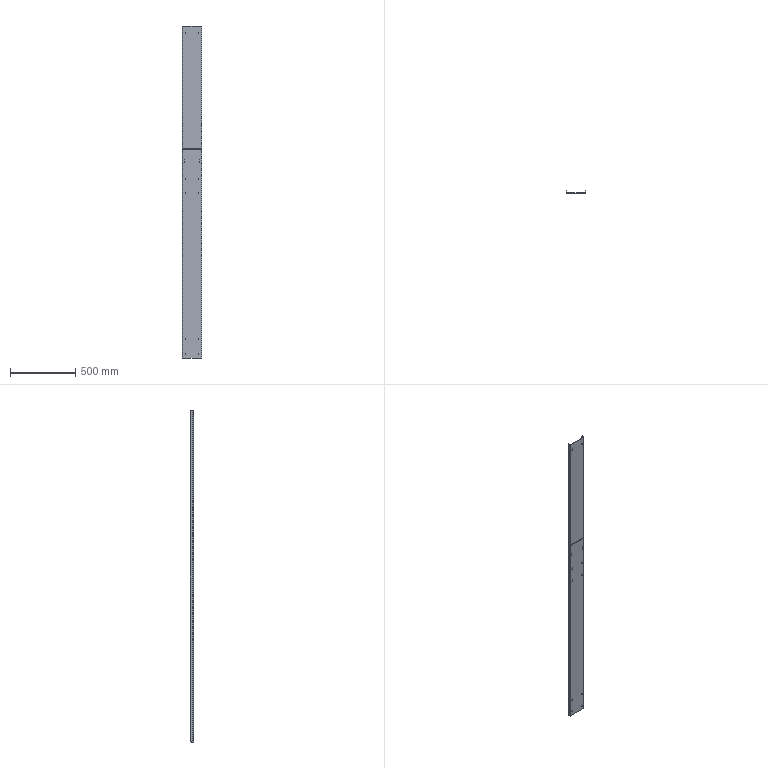Part | SolidWorks | features HoleWzd 3, Fillet 1, FlatPattern 1, SMBaseFlange 1, SheetMetal 1 | 1 solid | 80 faces | box 151 x 23 x 2540 mm | volume 1429422 mm3 | cylinder 42 | cone 20 | plane 18 | commonest cylinder face diameters 4.2 x34 10 x6 4 x2